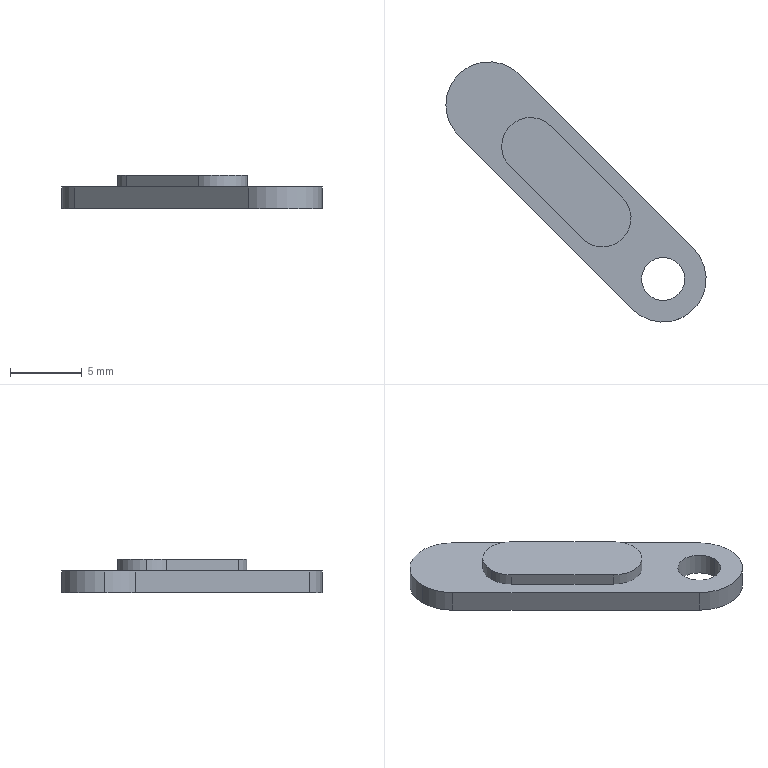Part | SolidWorks | features Cut 3, Extrusion 1, ICE 1 | 1 solid | 18 faces | box 18.138 x 18.138 x 2.3 mm | volume 212.007 mm3 | cylinder 10 | plane 8 | commonest cylinder face diameters 3 x4 4 x3 6 x3
STEP:
#1=CARTESIAN_POINT('',(-8.06,49.9,0.));
#2=VERTEX_POINT('',#1);
#3=CARTESIAN_POINT('',(-5.06,49.9,0.));
#4=VERTEX_POINT('',#3);
#5=CARTESIAN_POINT('',(-6.56,49.9,0.));
#6=DIRECTION('',(0.,0.,1.));
#7=DIRECTION('',(1.,0.,0.));
#8=AXIS2_PLACEMENT_3D('',#5,#6,#7);
#9=CIRCLE('',#8,1.5);
#10=EDGE_CURVE('',#2,#4,#9,.T.);
#11=ORIENTED_EDGE('',*,*,#10,.F.);
#12=CARTESIAN_POINT('',(-8.06,49.9,1.));
#13=VERTEX_POINT('',#12);
#14=CARTESIAN_POINT('',(-8.06,49.9,-12.));
#15=DIRECTION('',(0.,0.,1.));
#16=VECTOR('',#15,1000.);
#17=LINE('',#14,#16);
#18=EDGE_CURVE('',#2,#13,#17,.T.);
#19=ORIENTED_EDGE('',*,*,#18,.T.);
#20=CARTESIAN_POINT('',(-5.06,49.9,1.));
#21=VERTEX_POINT('',#20);
#22=CARTESIAN_POINT('',(-6.56,49.9,1.));
#23=DIRECTION('',(0.,0.,1.));
#24=DIRECTION('',(1.,0.,0.));
#25=AXIS2_PLACEMENT_3D('',#22,#23,#24);
#26=CIRCLE('',#25,1.5);
#27=EDGE_CURVE('',#13,#21,#26,.T.);
#28=ORIENTED_EDGE('',*,*,#27,.T.);
#29=CARTESIAN_POINT('',(-5.06,49.9,-12.));
#30=DIRECTION('',(0.,0.,1.));
#31=VECTOR('',#30,1000.);
#32=LINE('',#29,#31);
#33=EDGE_CURVE('',#4,#21,#32,.T.);
#34=ORIENTED_EDGE('',*,*,#33,.F.);
#35=EDGE_LOOP('',(#11,#19,#28,#34));
#36=FACE_OUTER_BOUND('',#35,.T.);
#37=CARTESIAN_POINT('',(-6.56,49.9,-12.));
#38=DIRECTION('',(0.,0.,1.));
#39=DIRECTION('',(1.,0.,0.));
#40=AXIS2_PLACEMENT_3D('',#37,#38,#39);
#41=CYLINDRICAL_SURFACE('',#40,1.5);
#42=ADVANCED_FACE('',(#36),#41,.F.);
#43=CARTESIAN_POINT('',(4.079,37.762,1.5));
#44=VERTEX_POINT('',#43);
#45=CARTESIAN_POINT('',(7.079,37.762,1.5));
#46=VERTEX_POINT('',#45);
#47=CARTESIAN_POINT('',(5.579,37.762,1.5));
#48=DIRECTION('',(0.,0.,1.));
#49=DIRECTION('',(1.,0.,0.));
#50=AXIS2_PLACEMENT_3D('',#47,#48,#49);
#51=CIRCLE('',#50,1.5);
#52=EDGE_CURVE('',#44,#46,#51,.T.);
#53=ORIENTED_EDGE('',*,*,#52,.T.);
#54=CARTESIAN_POINT('',(7.079,37.762,0.));
#55=VERTEX_POINT('',#54);
#56=CARTESIAN_POINT('',(7.079,37.762,0.8));
#57=DIRECTION('',(0.,0.,-1.));
#58=VECTOR('',#57,1000.);
#59=LINE('',#56,#58);
#60=EDGE_CURVE('',#46,#55,#59,.T.);
#61=ORIENTED_EDGE('',*,*,#60,.T.);
#62=CARTESIAN_POINT('',(4.079,37.762,0.));
#63=VERTEX_POINT('',#62);
#64=CARTESIAN_POINT('',(5.579,37.762,0.));
#65=DIRECTION('',(0.,0.,-1.));
#66=DIRECTION('',(-1.,0.,0.));
#67=AXIS2_PLACEMENT_3D('',#64,#65,#66);
#68=CIRCLE('',#67,1.5);
#69=EDGE_CURVE('',#55,#63,#68,.T.);
#70=ORIENTED_EDGE('',*,*,#69,.T.);
#71=CARTESIAN_POINT('',(4.079,37.762,0.8));
#72=DIRECTION('',(0.,0.,-1.));
#73=VECTOR('',#72,1000.);
#74=LINE('',#71,#73);
#75=EDGE_CURVE('',#44,#63,#74,.T.);
#76=ORIENTED_EDGE('',*,*,#75,.F.);
#77=EDGE_LOOP('',(#53,#61,#70,#76));
#78=FACE_OUTER_BOUND('',#77,.T.);
#79=CARTESIAN_POINT('',(5.579,37.762,0.8));
#80=DIRECTION('',(0.,0.,-1.));
#81=DIRECTION('',(-1.,0.,0.));
#82=AXIS2_PLACEMENT_3D('',#79,#80,#81);
#83=CYLINDRICAL_SURFACE('',#82,1.5);
#84=ADVANCED_FACE('',(#78),#83,.F.);
#85=CARTESIAN_POINT('',(-5.675,47.015,2.3));
#86=VERTEX_POINT('',#85);
#87=CARTESIAN_POINT('',(-5.089,45.601,2.3));
#88=VERTEX_POINT('',#87);
#89=CARTESIAN_POINT('',(-3.675,47.015,2.3));
#90=DIRECTION('',(0.,0.,1.));
#91=DIRECTION('',(1.,0.,0.));
#92=AXIS2_PLACEMENT_3D('',#89,#90,#91);
#93=CIRCLE('',#92,2.);
#94=EDGE_CURVE('',#86,#88,#93,.T.);
#95=ORIENTED_EDGE('',*,*,#94,.F.);
#96=CARTESIAN_POINT('',(-5.675,47.015,1.5));
#97=VERTEX_POINT('',#96);
#98=CARTESIAN_POINT('',(-5.675,47.015,2.3));
#99=DIRECTION('',(0.,0.,-1.));
#100=VECTOR('',#99,1000.);
#101=LINE('',#98,#100);
#102=EDGE_CURVE('',#86,#97,#101,.T.);
#103=ORIENTED_EDGE('',*,*,#102,.T.);
#104=CARTESIAN_POINT('',(-5.089,45.601,1.5));
#105=VERTEX_POINT('',#104);
#106=CARTESIAN_POINT('',(-3.675,47.015,1.5));
#107=DIRECTION('',(0.,0.,1.));
#108=DIRECTION('',(1.,0.,0.));
#109=AXIS2_PLACEMENT_3D('',#106,#107,#108);
#110=CIRCLE('',#109,2.);
#111=EDGE_CURVE('',#97,#105,#110,.T.);
#112=ORIENTED_EDGE('',*,*,#111,.T.);
#113=CARTESIAN_POINT('',(-5.089,45.601,2.3));
#114=DIRECTION('',(0.,0.,-1.));
#115=VECTOR('',#114,1000.);
#116=LINE('',#113,#115);
#117=EDGE_CURVE('',#88,#105,#116,.T.);
#118=ORIENTED_EDGE('',*,*,#117,.F.);
#119=EDGE_LOOP('',(#95,#103,#112,#118));
#120=FACE_OUTER_BOUND('',#119,.T.);
#121=CARTESIAN_POINT('',(-3.675,47.015,2.3));
#122=DIRECTION('',(0.,0.,-1.));
#123=DIRECTION('',(-1.,0.,0.));
#124=AXIS2_PLACEMENT_3D('',#121,#122,#123);
#125=CYLINDRICAL_SURFACE('',#124,2.);
#126=ADVANCED_FACE('',(#120),#125,.T.);
#127=CARTESIAN_POINT('',(-9.56,49.9,1.5));
#128=VERTEX_POINT('',#127);
#129=CARTESIAN_POINT('',(-8.681,47.779,1.5));
#130=VERTEX_POINT('',#129);
#131=CARTESIAN_POINT('',(-6.56,49.9,1.5));
#132=DIRECTION('',(0.,0.,1.));
#133=DIRECTION('',(1.,0.,0.));
#134=AXIS2_PLACEMENT_3D('',#131,#132,#133);
#135=CIRCLE('',#134,3.);
#136=EDGE_CURVE('',#128,#130,#135,.T.);
#137=ORIENTED_EDGE('',*,*,#136,.F.);
#138=CARTESIAN_POINT('',(-9.56,49.9,0.));
#139=VERTEX_POINT('',#138);
#140=CARTESIAN_POINT('',(-9.56,49.9,1.5));
#141=DIRECTION('',(0.,0.,-1.));
#142=VECTOR('',#141,1000.);
#143=LINE('',#140,#142);
#144=EDGE_CURVE('',#128,#139,#143,.T.);
#145=ORIENTED_EDGE('',*,*,#144,.T.);
#146=CARTESIAN_POINT('',(-8.681,47.779,0.));
#147=VERTEX_POINT('',#146);
#148=CARTESIAN_POINT('',(-6.56,49.9,0.));
#149=DIRECTION('',(0.,0.,1.));
#150=DIRECTION('',(1.,0.,0.));
#151=AXIS2_PLACEMENT_3D('',#148,#149,#150);
#152=CIRCLE('',#151,3.);
#153=EDGE_CURVE('',#139,#147,#152,.T.);
#154=ORIENTED_EDGE('',*,*,#153,.T.);
#155=CARTESIAN_POINT('',(-8.681,47.779,1.5));
#156=DIRECTION('',(0.,0.,-1.));
#157=VECTOR('',#156,1000.);
#158=LINE('',#155,#157);
#159=EDGE_CURVE('',#130,#147,#158,.T.);
#160=ORIENTED_EDGE('',*,*,#159,.F.);
#161=EDGE_LOOP('',(#137,#145,#154,#160));
#162=FACE_OUTER_BOUND('',#161,.T.);
#163=CARTESIAN_POINT('',(-6.56,49.9,1.5));
#164=DIRECTION('',(0.,0.,-1.));
#165=DIRECTION('',(-1.,0.,0.));
#166=AXIS2_PLACEMENT_3D('',#163,#164,#165);
#167=CYLINDRICAL_SURFACE('',#166,3.);
#168=ADVANCED_FACE('',(#162),#167,.T.);
#169=ORIENTED_EDGE('',*,*,#52,.F.);
#170=CARTESIAN_POINT('',(5.579,37.762,1.5));
#171=DIRECTION('',(0.,0.,1.));
#172=DIRECTION('',(1.,0.,0.));
#173=AXIS2_PLACEMENT_3D('',#170,#171,#172);
#174=CIRCLE('',#173,1.5);
#175=EDGE_CURVE('',#46,#44,#174,.T.);
#176=ORIENTED_EDGE('',*,*,#175,.F.);
#177=EDGE_LOOP('',(#169,#176));
#178=FACE_BOUND('',#177,.T.);
#179=CARTESIAN_POINT('',(3.457,35.64,1.5));
#180=VERTEX_POINT('',#179);
#181=CARTESIAN_POINT('',(7.7,39.883,1.5));
#182=VERTEX_POINT('',#181);
#183=CARTESIAN_POINT('',(5.579,37.762,1.5));
#184=DIRECTION('',(0.,0.,1.));
#185=DIRECTION('',(1.,0.,0.));
#186=AXIS2_PLACEMENT_3D('',#183,#184,#185);
#187=CIRCLE('',#186,3.);
#188=EDGE_CURVE('',#180,#182,#187,.T.);
#189=ORIENTED_EDGE('',*,*,#188,.T.);
#190=CARTESIAN_POINT('',(-4.439,52.022,1.5));
#191=VERTEX_POINT('',#190);
#192=CARTESIAN_POINT('',(7.7,39.883,1.5));
#193=DIRECTION('',(-0.7071,0.7071,0.));
#194=VECTOR('',#193,1000.);
#195=LINE('',#192,#194);
#196=EDGE_CURVE('',#182,#191,#195,.T.);
#197=ORIENTED_EDGE('',*,*,#196,.T.);
#198=CARTESIAN_POINT('',(-6.56,49.9,1.5));
#199=DIRECTION('',(0.,0.,1.));
#200=DIRECTION('',(1.,0.,0.));
#201=AXIS2_PLACEMENT_3D('',#198,#199,#200);
#202=CIRCLE('',#201,3.);
#203=EDGE_CURVE('',#191,#128,#202,.T.);
#204=ORIENTED_EDGE('',*,*,#203,.T.);
#205=ORIENTED_EDGE('',*,*,#136,.T.);
#206=CARTESIAN_POINT('',(3.457,35.64,1.5));
#207=DIRECTION('',(0.7071,-0.7071,0.));
#208=VECTOR('',#207,1000.);
#209=LINE('',#206,#208);
#210=EDGE_CURVE('',#130,#180,#209,.T.);
#211=ORIENTED_EDGE('',*,*,#210,.T.);
#212=EDGE_LOOP('',(#189,#197,#204,#205,#211));
#213=FACE_OUTER_BOUND('',#212,.T.);
#214=CARTESIAN_POINT('',(-0.06963,40.582,1.5));
#215=VERTEX_POINT('',#214);
#216=CARTESIAN_POINT('',(-5.089,45.601,1.5));
#217=DIRECTION('',(0.7071,-0.7071,0.));
#218=VECTOR('',#217,1000.);
#219=LINE('',#216,#218);
#220=EDGE_CURVE('',#105,#215,#219,.T.);
#221=ORIENTED_EDGE('',*,*,#220,.F.);
#222=ORIENTED_EDGE('',*,*,#111,.F.);
#223=CARTESIAN_POINT('',(-2.261,48.43,1.5));
#224=VERTEX_POINT('',#223);
#225=CARTESIAN_POINT('',(-3.675,47.015,1.5));
#226=DIRECTION('',(0.,0.,1.));
#227=DIRECTION('',(1.,0.,0.));
#228=AXIS2_PLACEMENT_3D('',#225,#226,#227);
#229=CIRCLE('',#228,2.);
#230=EDGE_CURVE('',#224,#97,#229,.T.);
#231=ORIENTED_EDGE('',*,*,#230,.F.);
#232=CARTESIAN_POINT('',(2.759,43.41,1.5));
#233=VERTEX_POINT('',#232);
#234=CARTESIAN_POINT('',(-2.261,48.43,1.5));
#235=DIRECTION('',(-0.7071,0.7071,0.));
#236=VECTOR('',#235,1000.);
#237=LINE('',#234,#236);
#238=EDGE_CURVE('',#233,#224,#237,.T.);
#239=ORIENTED_EDGE('',*,*,#238,.F.);
#240=CARTESIAN_POINT('',(1.345,41.996,1.5));
#241=DIRECTION('',(0.,0.,1.));
#242=DIRECTION('',(1.,0.,0.));
#243=AXIS2_PLACEMENT_3D('',#240,#241,#242);
#244=CIRCLE('',#243,2.);
#245=EDGE_CURVE('',#215,#233,#244,.T.);
#246=ORIENTED_EDGE('',*,*,#245,.F.);
#247=EDGE_LOOP('',(#221,#222,#231,#239,#246));
#248=FACE_BOUND('',#247,.T.);
#249=CARTESIAN_POINT('',(5.579,37.762,1.5));
#250=DIRECTION('',(0.,0.,1.));
#251=DIRECTION('',(1.,0.,0.));
#252=AXIS2_PLACEMENT_3D('',#249,#250,#251);
#253=PLANE('',#252);
#254=ADVANCED_FACE('',(#178,#213,#248),#253,.T.);
#255=CARTESIAN_POINT('',(3.457,35.64,0.));
#256=VERTEX_POINT('',#255);
#257=CARTESIAN_POINT('',(7.7,39.883,0.));
#258=VERTEX_POINT('',#257);
#259=CARTESIAN_POINT('',(5.579,37.762,0.));
#260=DIRECTION('',(0.,0.,1.));
#261=DIRECTION('',(1.,0.,0.));
#262=AXIS2_PLACEMENT_3D('',#259,#260,#261);
#263=CIRCLE('',#262,3.);
#264=EDGE_CURVE('',#256,#258,#263,.T.);
#265=ORIENTED_EDGE('',*,*,#264,.T.);
#266=CARTESIAN_POINT('',(7.7,39.883,1.5));
#267=DIRECTION('',(0.,0.,-1.));
#268=VECTOR('',#267,1000.);
#269=LINE('',#266,#268);
#270=EDGE_CURVE('',#182,#258,#269,.T.);
#271=ORIENTED_EDGE('',*,*,#270,.F.);
#272=ORIENTED_EDGE('',*,*,#188,.F.);
#273=CARTESIAN_POINT('',(3.457,35.64,1.5));
#274=DIRECTION('',(0.,0.,-1.));
#275=VECTOR('',#274,1000.);
#276=LINE('',#273,#275);
#277=EDGE_CURVE('',#180,#256,#276,.T.);
#278=ORIENTED_EDGE('',*,*,#277,.T.);
#279=EDGE_LOOP('',(#265,#271,#272,#278));
#280=FACE_OUTER_BOUND('',#279,.T.);
#281=CARTESIAN_POINT('',(5.579,37.762,1.5));
#282=DIRECTION('',(0.,0.,-1.));
#283=DIRECTION('',(-1.,0.,0.));
#284=AXIS2_PLACEMENT_3D('',#281,#282,#283);
#285=CYLINDRICAL_SURFACE('',#284,3.);
#286=ADVANCED_FACE('',(#280),#285,.T.);
#287=CARTESIAN_POINT('',(-4.439,52.022,0.));
#288=VERTEX_POINT('',#287);
#289=CARTESIAN_POINT('',(7.7,39.883,0.));
#290=DIRECTION('',(-0.7071,0.7071,0.));
#291=VECTOR('',#290,1000.);
#292=LINE('',#289,#291);
#293=EDGE_CURVE('',#258,#288,#292,.T.);
#294=ORIENTED_EDGE('',*,*,#293,.T.);
#295=CARTESIAN_POINT('',(-4.439,52.022,1.5));
#296=DIRECTION('',(0.,0.,-1.));
#297=VECTOR('',#296,1000.);
#298=LINE('',#295,#297);
#299=EDGE_CURVE('',#191,#288,#298,.T.);
#300=ORIENTED_EDGE('',*,*,#299,.F.);
#301=ORIENTED_EDGE('',*,*,#196,.F.);
#302=ORIENTED_EDGE('',*,*,#270,.T.);
#303=EDGE_LOOP('',(#294,#300,#301,#302));
#304=FACE_OUTER_BOUND('',#303,.T.);
#305=CARTESIAN_POINT('',(7.7,39.883,1.5));
#306=DIRECTION('',(-0.7071,-0.7071,0.));
#307=DIRECTION('',(0.7071,-0.7071,0.));
#308=AXIS2_PLACEMENT_3D('',#305,#306,#307);
#309=PLANE('',#308);
#310=ADVANCED_FACE('',(#304),#309,.F.);
#311=ORIENTED_EDGE('',*,*,#144,.F.);
#312=ORIENTED_EDGE('',*,*,#203,.F.);
#313=ORIENTED_EDGE('',*,*,#299,.T.);
#314=CARTESIAN_POINT('',(-6.56,49.9,0.));
#315=DIRECTION('',(0.,0.,1.));
#316=DIRECTION('',(1.,0.,0.));
#317=AXIS2_PLACEMENT_3D('',#314,#315,#316);
#318=CIRCLE('',#317,3.);
#319=EDGE_CURVE('',#288,#139,#318,.T.);
#320=ORIENTED_EDGE('',*,*,#319,.T.);
#321=EDGE_LOOP('',(#311,#312,#313,#320));
#322=FACE_OUTER_BOUND('',#321,.T.);
#323=CARTESIAN_POINT('',(-6.56,49.9,1.5));
#324=DIRECTION('',(0.,0.,-1.));
#325=DIRECTION('',(-1.,0.,0.));
#326=AXIS2_PLACEMENT_3D('',#323,#324,#325);
#327=CYLINDRICAL_SURFACE('',#326,3.);
#328=ADVANCED_FACE('',(#322),#327,.T.);
#329=CARTESIAN_POINT('',(3.457,35.64,0.));
#330=DIRECTION('',(0.7071,-0.7071,0.));
#331=VECTOR('',#330,1000.);
#332=LINE('',#329,#331);
#333=EDGE_CURVE('',#147,#256,#332,.T.);
#334=ORIENTED_EDGE('',*,*,#333,.T.);
#335=ORIENTED_EDGE('',*,*,#277,.F.);
#336=ORIENTED_EDGE('',*,*,#210,.F.);
#337=ORIENTED_EDGE('',*,*,#159,.T.);
#338=EDGE_LOOP('',(#334,#335,#336,#337));
#339=FACE_OUTER_BOUND('',#338,.T.);
#340=CARTESIAN_POINT('',(3.457,35.64,1.5));
#341=DIRECTION('',(0.7071,0.7071,0.));
#342=DIRECTION('',(-0.7071,0.7071,0.));
#343=AXIS2_PLACEMENT_3D('',#340,#341,#342);
#344=PLANE('',#343);
#345=ADVANCED_FACE('',(#339),#344,.F.);
#346=CARTESIAN_POINT('',(-6.56,49.9,0.));
#347=DIRECTION('',(0.,0.,1.));
#348=DIRECTION('',(1.,0.,0.));
#349=AXIS2_PLACEMENT_3D('',#346,#347,#348);
#350=CIRCLE('',#349,1.5);
#351=EDGE_CURVE('',#4,#2,#350,.T.);
#352=ORIENTED_EDGE('',*,*,#351,.T.);
#353=ORIENTED_EDGE('',*,*,#10,.T.);
#354=EDGE_LOOP('',(#352,#353));
#355=FACE_BOUND('',#354,.T.);
#356=CARTESIAN_POINT('',(5.579,37.762,0.));
#357=DIRECTION('',(0.,0.,-1.));
#358=DIRECTION('',(-1.,0.,0.));
#359=AXIS2_PLACEMENT_3D('',#356,#357,#358);
#360=CIRCLE('',#359,1.5);
#361=EDGE_CURVE('',#63,#55,#360,.T.);
#362=ORIENTED_EDGE('',*,*,#361,.F.);
#363=ORIENTED_EDGE('',*,*,#69,.F.);
#364=EDGE_LOOP('',(#362,#363));
#365=FACE_BOUND('',#364,.T.);
#366=ORIENTED_EDGE('',*,*,#264,.F.);
#367=ORIENTED_EDGE('',*,*,#333,.F.);
#368=ORIENTED_EDGE('',*,*,#153,.F.);
#369=ORIENTED_EDGE('',*,*,#319,.F.);
#370=ORIENTED_EDGE('',*,*,#293,.F.);
#371=EDGE_LOOP('',(#366,#367,#368,#369,#370));
#372=FACE_OUTER_BOUND('',#371,.T.);
#373=CARTESIAN_POINT('',(5.579,37.762,0.));
#374=DIRECTION('',(0.,0.,1.));
#375=DIRECTION('',(1.,0.,0.));
#376=AXIS2_PLACEMENT_3D('',#373,#374,#375);
#377=PLANE('',#376);
#378=ADVANCED_FACE('',(#355,#365,#372),#377,.F.);
#379=ORIENTED_EDGE('',*,*,#102,.F.);
#380=CARTESIAN_POINT('',(-2.261,48.43,2.3));
#381=VERTEX_POINT('',#380);
#382=CARTESIAN_POINT('',(-3.675,47.015,2.3));
#383=DIRECTION('',(0.,0.,1.));
#384=DIRECTION('',(1.,0.,0.));
#385=AXIS2_PLACEMENT_3D('',#382,#383,#384);
#386=CIRCLE('',#385,2.);
#387=EDGE_CURVE('',#381,#86,#386,.T.);
#388=ORIENTED_EDGE('',*,*,#387,.F.);
#389=CARTESIAN_POINT('',(-2.261,48.43,2.3));
#390=DIRECTION('',(0.,0.,-1.));
#391=VECTOR('',#390,1000.);
#392=LINE('',#389,#391);
#393=EDGE_CURVE('',#381,#224,#392,.T.);
#394=ORIENTED_EDGE('',*,*,#393,.T.);
#395=ORIENTED_EDGE('',*,*,#230,.T.);
#396=EDGE_LOOP('',(#379,#388,#394,#395));
#397=FACE_OUTER_BOUND('',#396,.T.);
#398=CARTESIAN_POINT('',(-3.675,47.015,2.3));
#399=DIRECTION('',(0.,0.,-1.));
#400=DIRECTION('',(-1.,0.,0.));
#401=AXIS2_PLACEMENT_3D('',#398,#399,#400);
#402=CYLINDRICAL_SURFACE('',#401,2.);
#403=ADVANCED_FACE('',(#397),#402,.T.);
#404=ORIENTED_EDGE('',*,*,#220,.T.);
#405=CARTESIAN_POINT('',(-0.06963,40.582,2.3));
#406=VERTEX_POINT('',#405);
#407=CARTESIAN_POINT('',(-0.06963,40.582,2.3));
#408=DIRECTION('',(0.,0.,-1.));
#409=VECTOR('',#408,1000.);
#410=LINE('',#407,#409);
#411=EDGE_CURVE('',#406,#215,#410,.T.);
#412=ORIENTED_EDGE('',*,*,#411,.F.);
#413=CARTESIAN_POINT('',(-5.089,45.601,2.3));
#414=DIRECTION('',(0.7071,-0.7071,0.));
#415=VECTOR('',#414,1000.);
#416=LINE('',#413,#415);
#417=EDGE_CURVE('',#88,#406,#416,.T.);
#418=ORIENTED_EDGE('',*,*,#417,.F.);
#419=ORIENTED_EDGE('',*,*,#117,.T.);
#420=EDGE_LOOP('',(#404,#412,#418,#419));
#421=FACE_OUTER_BOUND('',#420,.T.);
#422=CARTESIAN_POINT('',(-5.089,45.601,2.3));
#423=DIRECTION('',(0.7071,0.7071,0.));
#424=DIRECTION('',(-0.7071,0.7071,0.));
#425=AXIS2_PLACEMENT_3D('',#422,#423,#424);
#426=PLANE('',#425);
#427=ADVANCED_FACE('',(#421),#426,.F.);
#428=ORIENTED_EDGE('',*,*,#245,.T.);
#429=CARTESIAN_POINT('',(2.759,43.41,2.3));
#430=VERTEX_POINT('',#429);
#431=CARTESIAN_POINT('',(2.759,43.41,2.3));
#432=DIRECTION('',(0.,0.,-1.));
#433=VECTOR('',#432,1000.);
#434=LINE('',#431,#433);
#435=EDGE_CURVE('',#430,#233,#434,.T.);
#436=ORIENTED_EDGE('',*,*,#435,.F.);
#437=CARTESIAN_POINT('',(1.345,41.996,2.3));
#438=DIRECTION('',(0.,0.,1.));
#439=DIRECTION('',(1.,0.,0.));
#440=AXIS2_PLACEMENT_3D('',#437,#438,#439);
#441=CIRCLE('',#440,2.);
#442=EDGE_CURVE('',#406,#430,#441,.T.);
#443=ORIENTED_EDGE('',*,*,#442,.F.);
#444=ORIENTED_EDGE('',*,*,#411,.T.);
#445=EDGE_LOOP('',(#428,#436,#443,#444));
#446=FACE_OUTER_BOUND('',#445,.T.);
#447=CARTESIAN_POINT('',(1.345,41.996,2.3));
#448=DIRECTION('',(0.,0.,-1.));
#449=DIRECTION('',(-1.,0.,0.));
#450=AXIS2_PLACEMENT_3D('',#447,#448,#449);
#451=CYLINDRICAL_SURFACE('',#450,2.);
#452=ADVANCED_FACE('',(#446),#451,.T.);
#453=ORIENTED_EDGE('',*,*,#238,.T.);
#454=ORIENTED_EDGE('',*,*,#393,.F.);
#455=CARTESIAN_POINT('',(-2.261,48.43,2.3));
#456=DIRECTION('',(-0.7071,0.7071,0.));
#457=VECTOR('',#456,1000.);
#458=LINE('',#455,#457);
#459=EDGE_CURVE('',#430,#381,#458,.T.);
#460=ORIENTED_EDGE('',*,*,#459,.F.);
#461=ORIENTED_EDGE('',*,*,#435,.T.);
#462=EDGE_LOOP('',(#453,#454,#460,#461));
#463=FACE_OUTER_BOUND('',#462,.T.);
#464=CARTESIAN_POINT('',(-2.261,48.43,2.3));
#465=DIRECTION('',(-0.7071,-0.7071,0.));
#466=DIRECTION('',(0.7071,-0.7071,0.));
#467=AXIS2_PLACEMENT_3D('',#464,#465,#466);
#468=PLANE('',#467);
#469=ADVANCED_FACE('',(#463),#468,.F.);
#470=ORIENTED_EDGE('',*,*,#387,.T.);
#471=ORIENTED_EDGE('',*,*,#94,.T.);
#472=ORIENTED_EDGE('',*,*,#417,.T.);
#473=ORIENTED_EDGE('',*,*,#442,.T.);
#474=ORIENTED_EDGE('',*,*,#459,.T.);
#475=EDGE_LOOP('',(#470,#471,#472,#473,#474));
#476=FACE_OUTER_BOUND('',#475,.T.);
#477=CARTESIAN_POINT('',(-3.675,47.015,2.3));
#478=DIRECTION('',(0.,0.,1.));
#479=DIRECTION('',(1.,0.,0.));
#480=AXIS2_PLACEMENT_3D('',#477,#478,#479);
#481=PLANE('',#480);
#482=ADVANCED_FACE('',(#476),#481,.T.);
#483=ORIENTED_EDGE('',*,*,#60,.F.);
#484=ORIENTED_EDGE('',*,*,#175,.T.);
#485=ORIENTED_EDGE('',*,*,#75,.T.);
#486=ORIENTED_EDGE('',*,*,#361,.T.);
#487=EDGE_LOOP('',(#483,#484,#485,#486));
#488=FACE_OUTER_BOUND('',#487,.T.);
#489=CARTESIAN_POINT('',(5.579,37.762,0.8));
#490=DIRECTION('',(0.,0.,-1.));
#491=DIRECTION('',(-1.,0.,0.));
#492=AXIS2_PLACEMENT_3D('',#489,#490,#491);
#493=CYLINDRICAL_SURFACE('',#492,1.5);
#494=ADVANCED_FACE('',(#488),#493,.F.);
#495=ORIENTED_EDGE('',*,*,#18,.F.);
#496=ORIENTED_EDGE('',*,*,#351,.F.);
#497=ORIENTED_EDGE('',*,*,#33,.T.);
#498=CARTESIAN_POINT('',(-6.56,49.9,1.));
#499=DIRECTION('',(0.,0.,1.));
#500=DIRECTION('',(1.,0.,0.));
#501=AXIS2_PLACEMENT_3D('',#498,#499,#500);
#502=CIRCLE('',#501,1.5);
#503=EDGE_CURVE('',#21,#13,#502,.T.);
#504=ORIENTED_EDGE('',*,*,#503,.T.);
#505=EDGE_LOOP('',(#495,#496,#497,#504));
#506=FACE_OUTER_BOUND('',#505,.T.);
#507=CARTESIAN_POINT('',(-6.56,49.9,-12.));
#508=DIRECTION('',(0.,0.,1.));
#509=DIRECTION('',(1.,0.,0.));
#510=AXIS2_PLACEMENT_3D('',#507,#508,#509);
#511=CYLINDRICAL_SURFACE('',#510,1.5);
#512=ADVANCED_FACE('',(#506),#511,.F.);
#513=ORIENTED_EDGE('',*,*,#503,.F.);
#514=ORIENTED_EDGE('',*,*,#27,.F.);
#515=EDGE_LOOP('',(#513,#514));
#516=FACE_OUTER_BOUND('',#515,.T.);
#517=CARTESIAN_POINT('',(-6.56,49.9,1.));
#518=DIRECTION('',(0.,0.,1.));
#519=DIRECTION('',(1.,0.,0.));
#520=AXIS2_PLACEMENT_3D('',#517,#518,#519);
#521=PLANE('',#520);
#522=ADVANCED_FACE('',(#516),#521,.F.);
#523=CLOSED_SHELL('',(#42,#84,#126,#168,#254,#286,#310,#328,#345,#378,#403,#427,#452,#469,#482,#494,#512,#522));
#524=MANIFOLD_SOLID_BREP('',#523);
#525=CARTESIAN_POINT('',(0.,0.,0.));
#526=DIRECTION('',(0.,0.,1.));
#527=DIRECTION('',(1.,0.,0.));
#528=AXIS2_PLACEMENT_3D('',#525,#526,#527);
#529=(LENGTH_UNIT()NAMED_UNIT(*)SI_UNIT(.MILLI.,.METRE.));
#530=UNCERTAINTY_MEASURE_WITH_UNIT(LENGTH_MEASURE(0.00001),#529,'','');
#531=(NAMED_UNIT(*)PLANE_ANGLE_UNIT()SI_UNIT($,.RADIAN.));
#532=(NAMED_UNIT(*)SI_UNIT($,.STERADIAN.)SOLID_ANGLE_UNIT());
#533=(GEOMETRIC_REPRESENTATION_CONTEXT(3)GLOBAL_UNCERTAINTY_ASSIGNED_CONTEXT((#530))GLOBAL_UNIT_ASSIGNED_CONTEXT((#529,#531,#532))REPRESENTATION_CONTEXT('',''));
#534=ADVANCED_BREP_SHAPE_REPRESENTATION('',(#524,#528),#533);